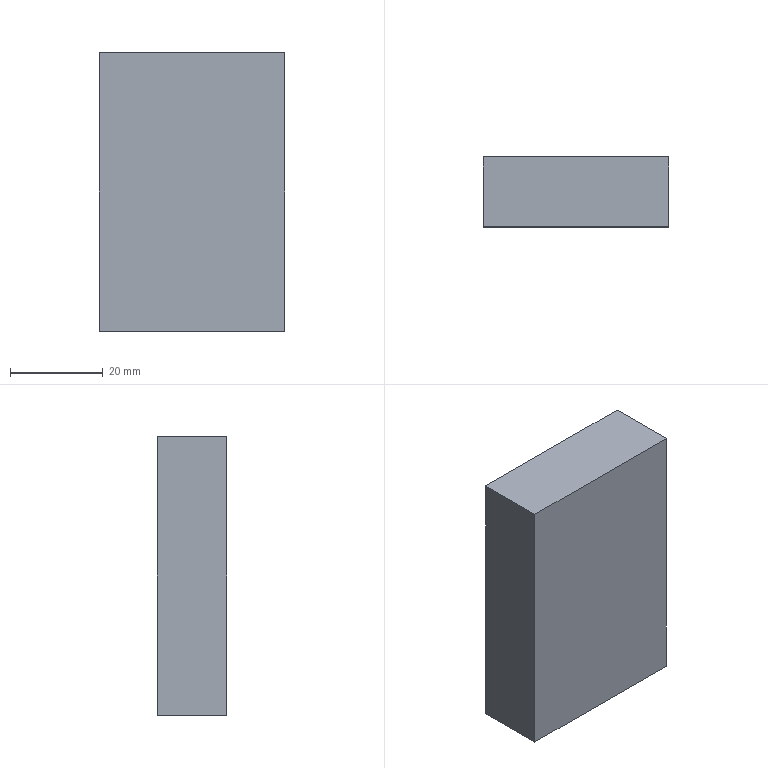Part | STEP file | Tube necking machine_id582_x_t | 1 solid | 6 faces | box 40 x 15 x 60 mm | volume 36000 mm3 | plane 6
STEP:
#1=CARTESIAN_POINT('',(0.,0.,0.));
#2=DIRECTION('',(0.,0.,1.));
#3=DIRECTION('',(1.,0.,0.));
#4=AXIS2_PLACEMENT_3D('',#1,#2,#3);
#5=CARTESIAN_POINT('',(290.5,95.,156.));
#6=VERTEX_POINT('',#5);
#7=CARTESIAN_POINT('',(250.5,95.,156.));
#8=VERTEX_POINT('',#7);
#9=CARTESIAN_POINT('',(305.5,95.,156.));
#10=DIRECTION('',(-1.,0.,0.));
#11=VECTOR('',#10,1.);
#12=LINE('',#9,#11);
#13=CARTESIAN_POINT('',(8.,0.,156.));
#14=DIRECTION('',(0.,0.,1.));
#15=DIRECTION('',(1.,0.,0.));
#16=AXIS2_PLACEMENT_3D('',#13,#14,#15);
#17=PLANE('',#16);
#18=CARTESIAN_POINT('',(297.5,95.));
#19=DIRECTION('',(-1.,0.));
#20=VECTOR('',#19,1.);
#21=LINE('',#18,#20);
#22=(GEOMETRIC_REPRESENTATION_CONTEXT(2)PARAMETRIC_REPRESENTATION_CONTEXT()REPRESENTATION_CONTEXT('',''));
#23=DEFINITIONAL_REPRESENTATION('',(#21),#22);
#24=PCURVE('',#17,#23);
#25=CARTESIAN_POINT('',(305.5,95.,252.));
#26=DIRECTION('',(0.,-1.,0.));
#27=DIRECTION('',(0.,0.,-1.));
#28=AXIS2_PLACEMENT_3D('',#25,#26,#27);
#29=PLANE('',#28);
#30=CARTESIAN_POINT('',(96.,0.));
#31=DIRECTION('',(0.,-1.));
#32=VECTOR('',#31,1.);
#33=LINE('',#30,#32);
#34=(GEOMETRIC_REPRESENTATION_CONTEXT(2)PARAMETRIC_REPRESENTATION_CONTEXT()REPRESENTATION_CONTEXT('',''));
#35=DEFINITIONAL_REPRESENTATION('',(#33),#34);
#36=PCURVE('',#29,#35);
#37=SURFACE_CURVE('',#12,(#24,#36),.PCURVE_S1.);
#38=EDGE_CURVE('',#6,#8,#37,.T.);
#39=ORIENTED_EDGE('',*,*,#38,.F.);
#40=CARTESIAN_POINT('',(290.5,80.,156.));
#41=VERTEX_POINT('',#40);
#42=CARTESIAN_POINT('',(290.5,0.,156.));
#43=DIRECTION('',(0.,-1.,0.));
#44=VECTOR('',#43,1.);
#45=LINE('',#42,#44);
#46=CARTESIAN_POINT('',(282.5,0.));
#47=DIRECTION('',(0.,-1.));
#48=VECTOR('',#47,1.);
#49=LINE('',#46,#48);
#50=(GEOMETRIC_REPRESENTATION_CONTEXT(2)PARAMETRIC_REPRESENTATION_CONTEXT()REPRESENTATION_CONTEXT('',''));
#51=DEFINITIONAL_REPRESENTATION('',(#49),#50);
#52=PCURVE('',#17,#51);
#53=CARTESIAN_POINT('',(290.5,50.,186.));
#54=DIRECTION('',(-1.,0.,0.));
#55=DIRECTION('',(0.,0.,1.));
#56=AXIS2_PLACEMENT_3D('',#53,#54,#55);
#57=PLANE('',#56);
#58=CARTESIAN_POINT('',(-30.,-50.));
#59=DIRECTION('',(0.,-1.));
#60=VECTOR('',#59,1.);
#61=LINE('',#58,#60);
#62=(GEOMETRIC_REPRESENTATION_CONTEXT(2)PARAMETRIC_REPRESENTATION_CONTEXT()REPRESENTATION_CONTEXT('',''));
#63=DEFINITIONAL_REPRESENTATION('',(#61),#62);
#64=PCURVE('',#57,#63);
#65=SURFACE_CURVE('',#45,(#52,#64),.PCURVE_S1.);
#66=EDGE_CURVE('',#6,#41,#65,.T.);
#67=ORIENTED_EDGE('',*,*,#66,.T.);
#68=CARTESIAN_POINT('',(250.5,80.,156.));
#69=VERTEX_POINT('',#68);
#70=CARTESIAN_POINT('',(8.,80.,156.));
#71=DIRECTION('',(1.,0.,0.));
#72=VECTOR('',#71,1.);
#73=LINE('',#70,#72);
#74=CARTESIAN_POINT('',(0.,80.));
#75=DIRECTION('',(1.,0.));
#76=VECTOR('',#75,1.);
#77=LINE('',#74,#76);
#78=(GEOMETRIC_REPRESENTATION_CONTEXT(2)PARAMETRIC_REPRESENTATION_CONTEXT()REPRESENTATION_CONTEXT('',''));
#79=DEFINITIONAL_REPRESENTATION('',(#77),#78);
#80=PCURVE('',#17,#79);
#81=CARTESIAN_POINT('',(290.5,80.,332.));
#82=DIRECTION('',(0.,-1.,0.));
#83=DIRECTION('',(0.,0.,-1.));
#84=AXIS2_PLACEMENT_3D('',#81,#82,#83);
#85=PLANE('',#84);
#86=CARTESIAN_POINT('',(176.,-282.5));
#87=DIRECTION('',(0.,1.));
#88=VECTOR('',#87,1.);
#89=LINE('',#86,#88);
#90=(GEOMETRIC_REPRESENTATION_CONTEXT(2)PARAMETRIC_REPRESENTATION_CONTEXT()REPRESENTATION_CONTEXT('',''));
#91=DEFINITIONAL_REPRESENTATION('',(#89),#90);
#92=PCURVE('',#85,#91);
#93=SURFACE_CURVE('',#73,(#80,#92),.PCURVE_S1.);
#94=EDGE_CURVE('',#69,#41,#93,.T.);
#95=ORIENTED_EDGE('',*,*,#94,.F.);
#96=CARTESIAN_POINT('',(250.5,0.,156.));
#97=DIRECTION('',(0.,1.,0.));
#98=VECTOR('',#97,1.);
#99=LINE('',#96,#98);
#100=CARTESIAN_POINT('',(242.5,0.));
#101=DIRECTION('',(0.,1.));
#102=VECTOR('',#101,1.);
#103=LINE('',#100,#102);
#104=(GEOMETRIC_REPRESENTATION_CONTEXT(2)PARAMETRIC_REPRESENTATION_CONTEXT()REPRESENTATION_CONTEXT('',''));
#105=DEFINITIONAL_REPRESENTATION('',(#103),#104);
#106=PCURVE('',#17,#105);
#107=CARTESIAN_POINT('',(250.5,50.,186.));
#108=DIRECTION('',(1.,0.,0.));
#109=DIRECTION('',(0.,0.,-1.));
#110=AXIS2_PLACEMENT_3D('',#107,#108,#109);
#111=PLANE('',#110);
#112=CARTESIAN_POINT('',(30.,-50.));
#113=DIRECTION('',(0.,1.));
#114=VECTOR('',#113,1.);
#115=LINE('',#112,#114);
#116=(GEOMETRIC_REPRESENTATION_CONTEXT(2)PARAMETRIC_REPRESENTATION_CONTEXT()REPRESENTATION_CONTEXT('',''));
#117=DEFINITIONAL_REPRESENTATION('',(#115),#116);
#118=PCURVE('',#111,#117);
#119=SURFACE_CURVE('',#99,(#106,#118),.PCURVE_S1.);
#120=EDGE_CURVE('',#69,#8,#119,.T.);
#121=ORIENTED_EDGE('',*,*,#120,.T.);
#122=EDGE_LOOP('',(#39,#67,#95,#121));
#123=FACE_BOUND('',#122,.T.);
#124=ADVANCED_FACE('',(#123),#17,.F.);
#125=CARTESIAN_POINT('',(290.5,95.,216.));
#126=VERTEX_POINT('',#125);
#127=CARTESIAN_POINT('',(290.5,80.,216.));
#128=VERTEX_POINT('',#127);
#129=CARTESIAN_POINT('',(290.5,0.,216.));
#130=DIRECTION('',(0.,-1.,0.));
#131=VECTOR('',#130,1.);
#132=LINE('',#129,#131);
#133=CARTESIAN_POINT('',(8.,0.,216.));
#134=DIRECTION('',(0.,0.,1.));
#135=DIRECTION('',(1.,0.,0.));
#136=AXIS2_PLACEMENT_3D('',#133,#134,#135);
#137=PLANE('',#136);
#138=CARTESIAN_POINT('',(282.5,0.));
#139=DIRECTION('',(0.,-1.));
#140=VECTOR('',#139,1.);
#141=LINE('',#138,#140);
#142=(GEOMETRIC_REPRESENTATION_CONTEXT(2)PARAMETRIC_REPRESENTATION_CONTEXT()REPRESENTATION_CONTEXT('',''));
#143=DEFINITIONAL_REPRESENTATION('',(#141),#142);
#144=PCURVE('',#137,#143);
#145=CARTESIAN_POINT('',(30.,-50.));
#146=DIRECTION('',(0.,-1.));
#147=VECTOR('',#146,1.);
#148=LINE('',#145,#147);
#149=(GEOMETRIC_REPRESENTATION_CONTEXT(2)PARAMETRIC_REPRESENTATION_CONTEXT()REPRESENTATION_CONTEXT('',''));
#150=DEFINITIONAL_REPRESENTATION('',(#148),#149);
#151=PCURVE('',#57,#150);
#152=SURFACE_CURVE('',#132,(#144,#151),.PCURVE_S1.);
#153=EDGE_CURVE('',#126,#128,#152,.T.);
#154=ORIENTED_EDGE('',*,*,#153,.F.);
#155=CARTESIAN_POINT('',(250.5,95.,216.));
#156=VERTEX_POINT('',#155);
#157=CARTESIAN_POINT('',(305.5,95.,216.));
#158=DIRECTION('',(-1.,0.,0.));
#159=VECTOR('',#158,1.);
#160=LINE('',#157,#159);
#161=CARTESIAN_POINT('',(297.5,95.));
#162=DIRECTION('',(-1.,0.));
#163=VECTOR('',#162,1.);
#164=LINE('',#161,#163);
#165=(GEOMETRIC_REPRESENTATION_CONTEXT(2)PARAMETRIC_REPRESENTATION_CONTEXT()REPRESENTATION_CONTEXT('',''));
#166=DEFINITIONAL_REPRESENTATION('',(#164),#165);
#167=PCURVE('',#137,#166);
#168=CARTESIAN_POINT('',(36.,0.));
#169=DIRECTION('',(0.,-1.));
#170=VECTOR('',#169,1.);
#171=LINE('',#168,#170);
#172=(GEOMETRIC_REPRESENTATION_CONTEXT(2)PARAMETRIC_REPRESENTATION_CONTEXT()REPRESENTATION_CONTEXT('',''));
#173=DEFINITIONAL_REPRESENTATION('',(#171),#172);
#174=PCURVE('',#29,#173);
#175=SURFACE_CURVE('',#160,(#167,#174),.PCURVE_S1.);
#176=EDGE_CURVE('',#126,#156,#175,.T.);
#177=ORIENTED_EDGE('',*,*,#176,.T.);
#178=CARTESIAN_POINT('',(250.5,80.,216.));
#179=VERTEX_POINT('',#178);
#180=CARTESIAN_POINT('',(250.5,0.,216.));
#181=DIRECTION('',(0.,1.,0.));
#182=VECTOR('',#181,1.);
#183=LINE('',#180,#182);
#184=CARTESIAN_POINT('',(242.5,0.));
#185=DIRECTION('',(0.,1.));
#186=VECTOR('',#185,1.);
#187=LINE('',#184,#186);
#188=(GEOMETRIC_REPRESENTATION_CONTEXT(2)PARAMETRIC_REPRESENTATION_CONTEXT()REPRESENTATION_CONTEXT('',''));
#189=DEFINITIONAL_REPRESENTATION('',(#187),#188);
#190=PCURVE('',#137,#189);
#191=CARTESIAN_POINT('',(-30.,-50.));
#192=DIRECTION('',(0.,1.));
#193=VECTOR('',#192,1.);
#194=LINE('',#191,#193);
#195=(GEOMETRIC_REPRESENTATION_CONTEXT(2)PARAMETRIC_REPRESENTATION_CONTEXT()REPRESENTATION_CONTEXT('',''));
#196=DEFINITIONAL_REPRESENTATION('',(#194),#195);
#197=PCURVE('',#111,#196);
#198=SURFACE_CURVE('',#183,(#190,#197),.PCURVE_S1.);
#199=EDGE_CURVE('',#179,#156,#198,.T.);
#200=ORIENTED_EDGE('',*,*,#199,.F.);
#201=CARTESIAN_POINT('',(8.,80.,216.));
#202=DIRECTION('',(1.,0.,0.));
#203=VECTOR('',#202,1.);
#204=LINE('',#201,#203);
#205=CARTESIAN_POINT('',(0.,80.));
#206=DIRECTION('',(1.,0.));
#207=VECTOR('',#206,1.);
#208=LINE('',#205,#207);
#209=(GEOMETRIC_REPRESENTATION_CONTEXT(2)PARAMETRIC_REPRESENTATION_CONTEXT()REPRESENTATION_CONTEXT('',''));
#210=DEFINITIONAL_REPRESENTATION('',(#208),#209);
#211=PCURVE('',#137,#210);
#212=CARTESIAN_POINT('',(116.,-282.5));
#213=DIRECTION('',(0.,1.));
#214=VECTOR('',#213,1.);
#215=LINE('',#212,#214);
#216=(GEOMETRIC_REPRESENTATION_CONTEXT(2)PARAMETRIC_REPRESENTATION_CONTEXT()REPRESENTATION_CONTEXT('',''));
#217=DEFINITIONAL_REPRESENTATION('',(#215),#216);
#218=PCURVE('',#85,#217);
#219=SURFACE_CURVE('',#204,(#211,#218),.PCURVE_S1.);
#220=EDGE_CURVE('',#179,#128,#219,.T.);
#221=ORIENTED_EDGE('',*,*,#220,.T.);
#222=EDGE_LOOP('',(#154,#177,#200,#221));
#223=FACE_BOUND('',#222,.T.);
#224=ADVANCED_FACE('',(#223),#137,.T.);
#225=ORIENTED_EDGE('',*,*,#176,.F.);
#226=CARTESIAN_POINT('',(290.5,95.,252.));
#227=DIRECTION('',(0.,0.,-1.));
#228=VECTOR('',#227,1.);
#229=LINE('',#226,#228);
#230=CARTESIAN_POINT('',(0.,-15.));
#231=DIRECTION('',(1.,0.));
#232=VECTOR('',#231,1.);
#233=LINE('',#230,#232);
#234=(GEOMETRIC_REPRESENTATION_CONTEXT(2)PARAMETRIC_REPRESENTATION_CONTEXT()REPRESENTATION_CONTEXT('',''));
#235=DEFINITIONAL_REPRESENTATION('',(#233),#234);
#236=PCURVE('',#29,#235);
#237=CARTESIAN_POINT('',(66.,45.));
#238=DIRECTION('',(-1.,0.));
#239=VECTOR('',#238,1.);
#240=LINE('',#237,#239);
#241=(GEOMETRIC_REPRESENTATION_CONTEXT(2)PARAMETRIC_REPRESENTATION_CONTEXT()REPRESENTATION_CONTEXT('',''));
#242=DEFINITIONAL_REPRESENTATION('',(#240),#241);
#243=PCURVE('',#57,#242);
#244=SURFACE_CURVE('',#229,(#236,#243),.PCURVE_S1.);
#245=EDGE_CURVE('',#126,#6,#244,.T.);
#246=ORIENTED_EDGE('',*,*,#245,.T.);
#247=ORIENTED_EDGE('',*,*,#38,.T.);
#248=CARTESIAN_POINT('',(250.5,95.,252.));
#249=DIRECTION('',(0.,0.,1.));
#250=VECTOR('',#249,1.);
#251=LINE('',#248,#250);
#252=CARTESIAN_POINT('',(0.,-55.));
#253=DIRECTION('',(-1.,0.));
#254=VECTOR('',#253,1.);
#255=LINE('',#252,#254);
#256=(GEOMETRIC_REPRESENTATION_CONTEXT(2)PARAMETRIC_REPRESENTATION_CONTEXT()REPRESENTATION_CONTEXT('',''));
#257=DEFINITIONAL_REPRESENTATION('',(#255),#256);
#258=PCURVE('',#29,#257);
#259=CARTESIAN_POINT('',(-66.,45.));
#260=DIRECTION('',(-1.,0.));
#261=VECTOR('',#260,1.);
#262=LINE('',#259,#261);
#263=(GEOMETRIC_REPRESENTATION_CONTEXT(2)PARAMETRIC_REPRESENTATION_CONTEXT()REPRESENTATION_CONTEXT('',''));
#264=DEFINITIONAL_REPRESENTATION('',(#262),#263);
#265=PCURVE('',#111,#264);
#266=SURFACE_CURVE('',#251,(#258,#265),.PCURVE_S1.);
#267=EDGE_CURVE('',#8,#156,#266,.T.);
#268=ORIENTED_EDGE('',*,*,#267,.T.);
#269=EDGE_LOOP('',(#225,#246,#247,#268));
#270=FACE_BOUND('',#269,.T.);
#271=ADVANCED_FACE('',(#270),#29,.F.);
#272=CARTESIAN_POINT('',(250.5,80.,332.));
#273=DIRECTION('',(0.,0.,1.));
#274=VECTOR('',#273,1.);
#275=LINE('',#272,#274);
#276=CARTESIAN_POINT('',(0.,-40.));
#277=DIRECTION('',(-1.,0.));
#278=VECTOR('',#277,1.);
#279=LINE('',#276,#278);
#280=(GEOMETRIC_REPRESENTATION_CONTEXT(2)PARAMETRIC_REPRESENTATION_CONTEXT()REPRESENTATION_CONTEXT('',''));
#281=DEFINITIONAL_REPRESENTATION('',(#279),#280);
#282=PCURVE('',#85,#281);
#283=CARTESIAN_POINT('',(-146.,30.));
#284=DIRECTION('',(-1.,0.));
#285=VECTOR('',#284,1.);
#286=LINE('',#283,#285);
#287=(GEOMETRIC_REPRESENTATION_CONTEXT(2)PARAMETRIC_REPRESENTATION_CONTEXT()REPRESENTATION_CONTEXT('',''));
#288=DEFINITIONAL_REPRESENTATION('',(#286),#287);
#289=PCURVE('',#111,#288);
#290=SURFACE_CURVE('',#275,(#282,#289),.PCURVE_S1.);
#291=EDGE_CURVE('',#69,#179,#290,.T.);
#292=ORIENTED_EDGE('',*,*,#291,.F.);
#293=ORIENTED_EDGE('',*,*,#94,.T.);
#294=CARTESIAN_POINT('',(290.5,80.,332.));
#295=DIRECTION('',(0.,0.,1.));
#296=VECTOR('',#295,1.);
#297=LINE('',#294,#296);
#298=CARTESIAN_POINT('',(0.,0.));
#299=DIRECTION('',(-1.,0.));
#300=VECTOR('',#299,1.);
#301=LINE('',#298,#300);
#302=(GEOMETRIC_REPRESENTATION_CONTEXT(2)PARAMETRIC_REPRESENTATION_CONTEXT()REPRESENTATION_CONTEXT('',''));
#303=DEFINITIONAL_REPRESENTATION('',(#301),#302);
#304=PCURVE('',#85,#303);
#305=CARTESIAN_POINT('',(146.,30.));
#306=DIRECTION('',(1.,0.));
#307=VECTOR('',#306,1.);
#308=LINE('',#305,#307);
#309=(GEOMETRIC_REPRESENTATION_CONTEXT(2)PARAMETRIC_REPRESENTATION_CONTEXT()REPRESENTATION_CONTEXT('',''));
#310=DEFINITIONAL_REPRESENTATION('',(#308),#309);
#311=PCURVE('',#57,#310);
#312=SURFACE_CURVE('',#297,(#304,#311),.PCURVE_S1.);
#313=EDGE_CURVE('',#41,#128,#312,.T.);
#314=ORIENTED_EDGE('',*,*,#313,.T.);
#315=ORIENTED_EDGE('',*,*,#220,.F.);
#316=EDGE_LOOP('',(#292,#293,#314,#315));
#317=FACE_BOUND('',#316,.T.);
#318=ADVANCED_FACE('',(#317),#85,.T.);
#319=ORIENTED_EDGE('',*,*,#120,.F.);
#320=ORIENTED_EDGE('',*,*,#291,.T.);
#321=ORIENTED_EDGE('',*,*,#199,.T.);
#322=ORIENTED_EDGE('',*,*,#267,.F.);
#323=EDGE_LOOP('',(#319,#320,#321,#322));
#324=FACE_BOUND('',#323,.T.);
#325=ADVANCED_FACE('',(#324),#111,.F.);
#326=ORIENTED_EDGE('',*,*,#313,.F.);
#327=ORIENTED_EDGE('',*,*,#66,.F.);
#328=ORIENTED_EDGE('',*,*,#245,.F.);
#329=ORIENTED_EDGE('',*,*,#153,.T.);
#330=EDGE_LOOP('',(#326,#327,#328,#329));
#331=FACE_BOUND('',#330,.T.);
#332=ADVANCED_FACE('',(#331),#57,.F.);
#333=CLOSED_SHELL('',(#124,#224,#271,#318,#325,#332));
#334=MANIFOLD_SOLID_BREP('',#333);
#335=(LENGTH_UNIT()NAMED_UNIT(*)SI_UNIT(.MILLI.,.METRE.));
#336=UNCERTAINTY_MEASURE_WITH_UNIT(LENGTH_MEASURE(0.0000001),#335,'','');
#337=(NAMED_UNIT(*)PLANE_ANGLE_UNIT()SI_UNIT($,.RADIAN.));
#338=(NAMED_UNIT(*)SI_UNIT($,.STERADIAN.)SOLID_ANGLE_UNIT());
#339=(GEOMETRIC_REPRESENTATION_CONTEXT(3)GLOBAL_UNCERTAINTY_ASSIGNED_CONTEXT((#336))GLOBAL_UNIT_ASSIGNED_CONTEXT((#335,#337,#338))REPRESENTATION_CONTEXT('',''));
#340=ADVANCED_BREP_SHAPE_REPRESENTATION('',(#4,#334),#339);